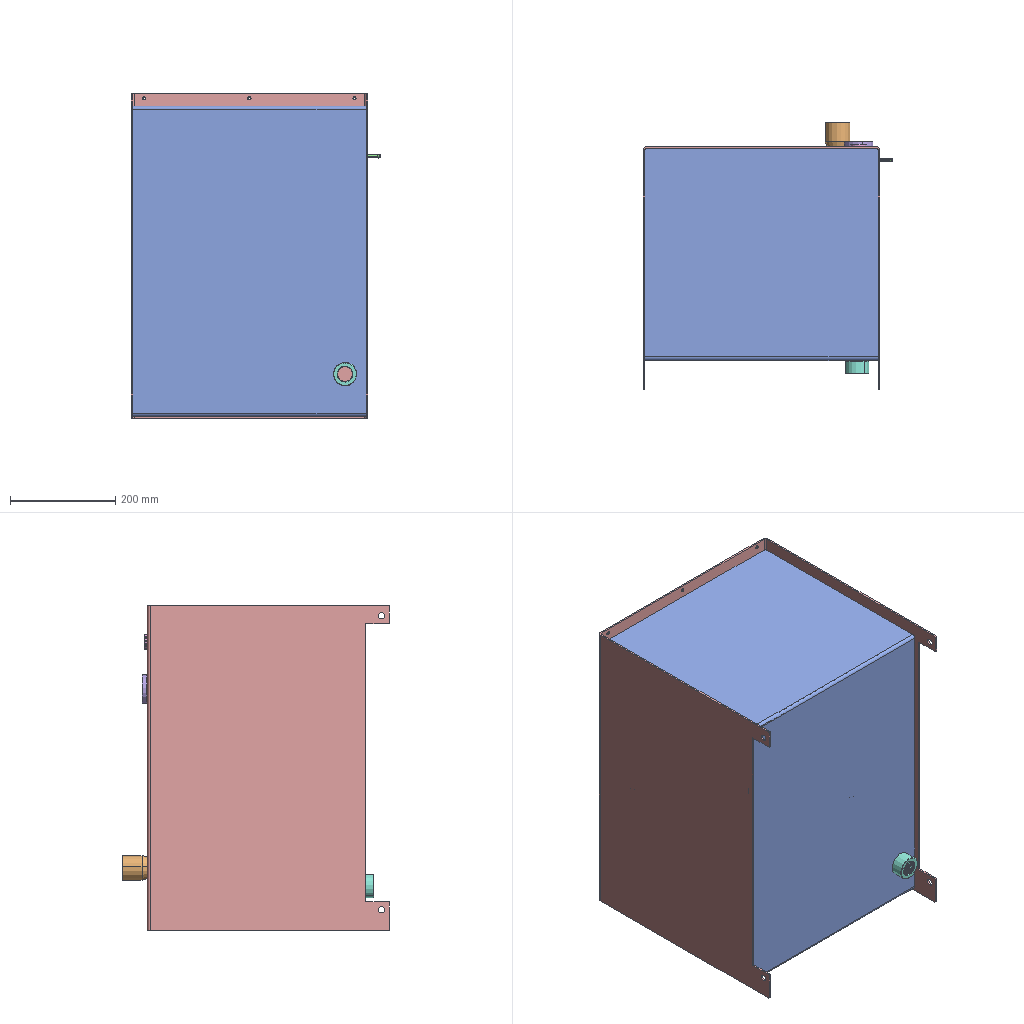Assembly | SolidWorks | 8 different items | 8 placed | box 475 x 508 x 620 mm
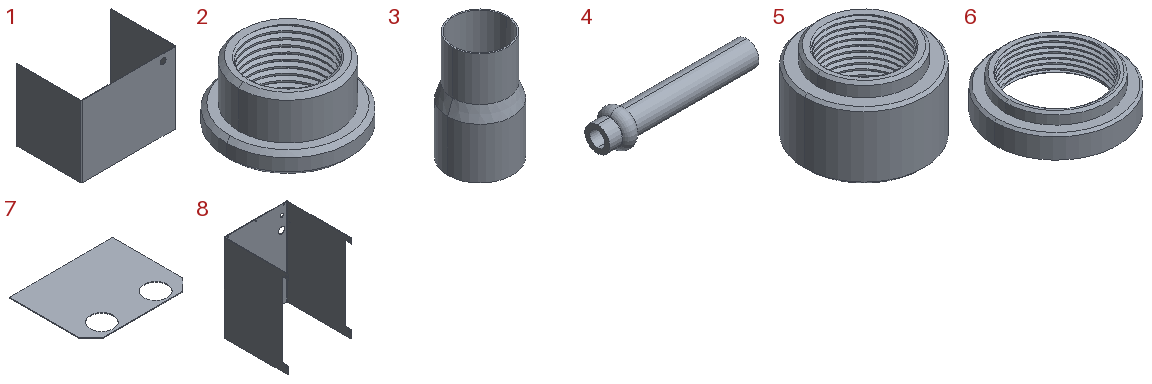Parts list (item | quantity | size | volume | features):
1 | x1 | 590 x 403 x 444 mm | 1843422 mm3 | features Fillet 1, FlatPattern 1, ICE 1, SMBaseFlange 1, SheetMetal 1
2 | x1 | 30 x 30 x 15 mm | 3564 mm3 | features ICE 2, Chamfer 1, Extrusion 1, SweepThread 1
3 | x1 | 47 x 47 x 79 mm | 10603 mm3 | features 3DProfileFeature 2, ICE 2, NetBlend 1, NetBlendCut 1
4 | x1 | 30 x 7 x 7 mm | 414.784 mm3 | features Fillet 1, Revolution 1
5 | x1 | 45 x 45 x 30 mm | 24610 mm3 | features Chamfer 2, ICE 2, Extrusion 1, SweepThread 1
6 | x1 | 55 x 55 x 15 mm | 12694 mm3 | features Chamfer 1, Extrusion 1, ICE 1, SweepThread 1
7 | x1 | 444 x 350 x 3 mm | 411576 mm3 | features Extrusion 1
8 | x1 | 450 x 461 x 620 mm | 2378784 mm3 | features ICE 3, Fillet 1, FlatPattern 1, LPattern 1, SMBaseFlange 1, SheetMetal 1, SweepThread 1
Mates (type | each side: item.copy, entity, surface, feature):
Coincident | 8.1 face plane Base-Flange1 | 1.1 face plane Base-Flange1 | 2 times
DistanceDim | 1.1 face plane Base-Flange1 | 8.1 face plane Base-Flange1
Coincident | 8.1 face plane Base-Flange1 | 7.1 face plane Boss-Extrude1
DistanceDim | 7.1 face plane Boss-Extrude1 | 1.1 face plane Base-Flange1
Coincident | 1.1 face plane Base-Flange1 | 7.1 face plane Boss-Extrude1
Concentric | 8.1 edge | 2.1 edge
Coincident | 8.1 face plane Base-Flange1 | 2.1 face plane Cut-Extrude1
Coincident | 1.1 face plane Base-Flange1 | 5.1 face plane Cut-Extrude1
Concentric | 1.1 edge | 5.1 edge
Concentric | 8.1 edge | 3.1 edge
Coincident | 8.1 face plane Base-Flange1 | 3.1 edge
Coincident | 8.1 face plane Base-Flange1 | 6.1 face plane Boss-Extrude1
Concentric | 8.1 edge | 6.1 face cylinder Boss-Extrude1
Concentric | 8.1 face cylinder Cut-Extrude4 | 4.1 face cylinder Revolve1
DistanceDim | 4.1 face plane Revolve1 | 8.1 face plane Base-Flange1